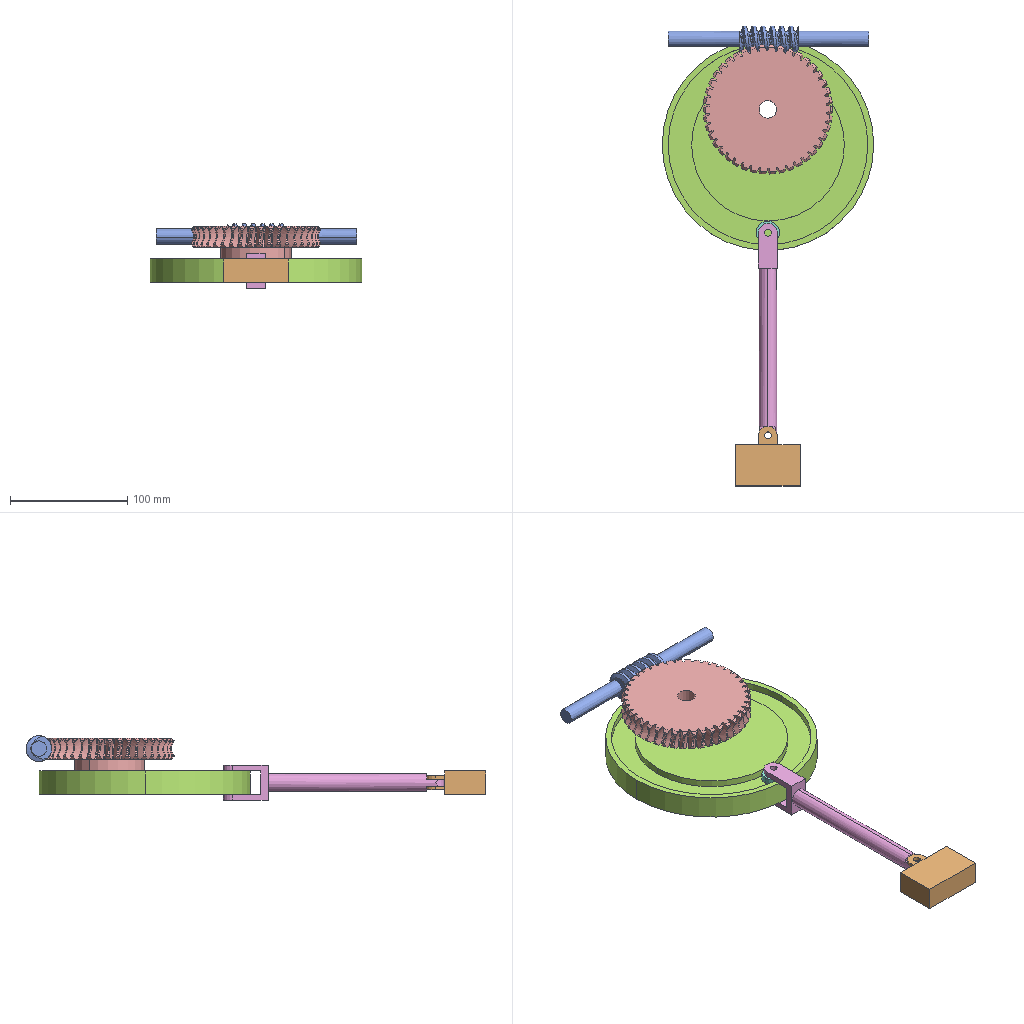Assembly | SolidWorks | 6 different items | 7 placed | box 180 x 392 x 55 mm
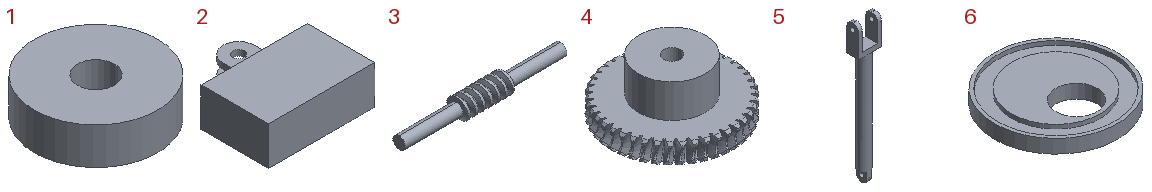Parts list (item | quantity | size | volume | features):
1 | x2 | 20 x 20 x 6 mm | 1715 mm3 | features Extrusion 1
2 | x1 | 55 x 51 x 20 mm | 39702 mm3 | features ICE 3, Extrusion 1
3 | x1 | 171 x 22 x 22 mm | 28864 mm3 | features ICE 3, Helix 1, RefAxis 1, Revolution 1, SweepCut 1
4 | x1 | 110.006 x 109.957 x 48 mm | 224193 mm3 | features ICE 2, CirPattern 1, Helix 1, RefAxis 1, Revolution 1, SweepCut 1
5 | x1 | 30 x 16 x 188 mm | 32315 mm3 | features ICE 5, Extrusion 1
6 | x1 | 180 x 180 x 20 mm | 339292 mm3 | features ICE 2, Extrusion 1
Mates (type | each side: item.copy, entity, surface, feature):
Concentric | 5.1 face cylinder Cut-Extrude2 | 1.1 face cylinder Boss-Extrude1
Coincident | 5.1 face plane Cut-Extrude1 | 1.1 face plane Boss-Extrude1
Concentric | 5.1 face cylinder Cut-Extrude2 | 1.2 face cylinder Boss-Extrude1
Coincident | 5.1 face plane Cut-Extrude1 | 1.2 face plane Boss-Extrude1
Tangent | 6.1 face cylinder Cut-Extrude1 | 1.2 face cylinder Boss-Extrude1
Coincident | 6.1 face plane Boss-Extrude1 | 5.1 face plane Cut-Extrude1
Concentric | 3.1 face cylinder Boss-Extrude1 | assembly select_type:10
Coincident | 4.1 select_type:24 | assembly select_type:11
DistanceDim | 4.1 face plane Revolve1 | assembly plane
DistanceDim | assembly select_type:10 | 3.1 face plane Boss-Extrude3
GearDim | 4.1 face cone Revolve1 | 3.1 face cylinder Revolve1
Concentric | 4.1 face cylinder Boss-Extrude1 | 6.1 face cylinder Boss-Extrude1
Coincident | 4.1 face plane Boss-Extrude1 | 6.1 face plane Boss-Extrude1
Parallel | 5.1 face cylinder Boss-Extrude1 | assembly select_type:10
DistanceDim | 5.1 face cylinder Boss-Extrude1 | 3.1 face plane Boss-Extrude3
Concentric | 5.1 face cylinder Cut-Extrude4 | 2.1 face cylinder Cut-Extrude2
Coincident | 5.1 face plane Cut-Extrude3 | 2.1 face plane Cut-Extrude1
Parallel | 3.1 face plane Boss-Extrude3 | 2.1 face plane Boss-Extrude1